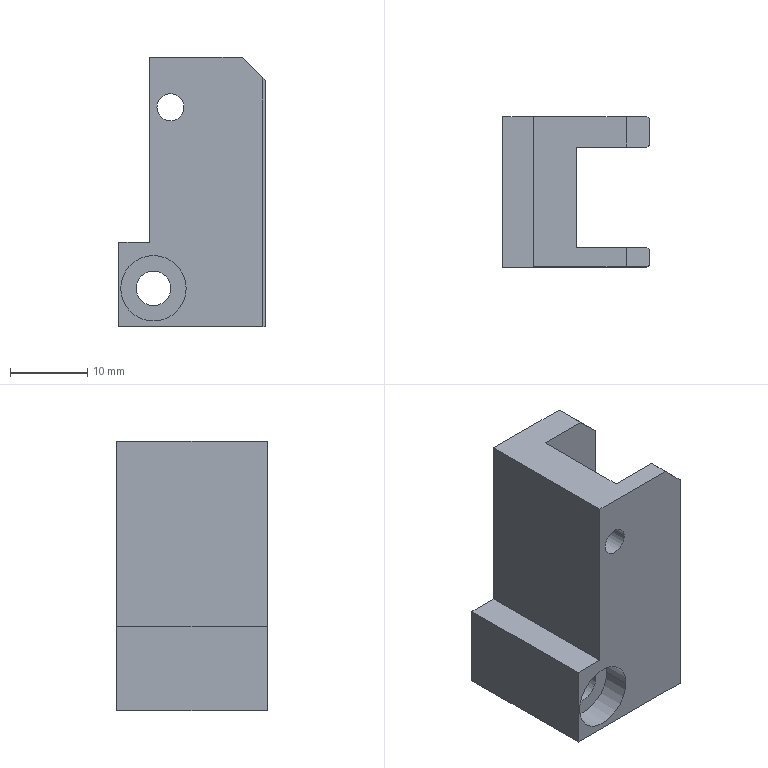Part | NX | 1 solid | 25 faces | box 19 x 19.5 x 35 mm | volume 6098 mm3 | plane 19 | cylinder 6 | commonest cylinder face diameters 3.5 x2 4.5 x2 8.5 x2
STEP:
#1=CARTESIAN_POINT('',(9.5,16.462,0.));
#2=VERTEX_POINT('',#1);
#3=CARTESIAN_POINT('',(18.7,16.462,0.));
#4=VERTEX_POINT('',#3);
#5=CARTESIAN_POINT('',(0.,16.462,0.));
#6=DIRECTION('',(1.,0.,0.));
#7=VECTOR('',#6,1000.);
#8=LINE('',#5,#7);
#9=EDGE_CURVE('',#2,#4,#8,.T.);
#10=ORIENTED_EDGE('',*,*,#9,.F.);
#11=CARTESIAN_POINT('',(9.5,3.462,0.));
#12=VERTEX_POINT('',#11);
#13=CARTESIAN_POINT('',(9.5,0.,0.));
#14=DIRECTION('',(0.,1.,0.));
#15=VECTOR('',#14,1000.);
#16=LINE('',#13,#15);
#17=EDGE_CURVE('',#12,#2,#16,.T.);
#18=ORIENTED_EDGE('',*,*,#17,.F.);
#19=CARTESIAN_POINT('',(18.7,3.462,0.));
#20=VERTEX_POINT('',#19);
#21=CARTESIAN_POINT('',(0.,3.462,0.));
#22=DIRECTION('',(-1.,0.,0.));
#23=VECTOR('',#22,1000.);
#24=LINE('',#21,#23);
#25=EDGE_CURVE('',#20,#12,#24,.T.);
#26=ORIENTED_EDGE('',*,*,#25,.F.);
#27=CARTESIAN_POINT('',(19.,3.162,0.));
#28=VERTEX_POINT('',#27);
#29=CARTESIAN_POINT('',(0.,22.162,0.));
#30=DIRECTION('',(0.7071,-0.7071,0.));
#31=VECTOR('',#30,1000.);
#32=LINE('',#29,#31);
#33=EDGE_CURVE('',#20,#28,#32,.T.);
#34=ORIENTED_EDGE('',*,*,#33,.T.);
#35=CARTESIAN_POINT('',(19.,1.212,0.));
#36=VERTEX_POINT('',#35);
#37=CARTESIAN_POINT('',(19.,0.,0.));
#38=DIRECTION('',(0.,-1.,0.));
#39=VECTOR('',#38,1000.);
#40=LINE('',#37,#39);
#41=EDGE_CURVE('',#28,#36,#40,.T.);
#42=ORIENTED_EDGE('',*,*,#41,.T.);
#43=CARTESIAN_POINT('',(18.7,0.912,0.));
#44=VERTEX_POINT('',#43);
#45=CARTESIAN_POINT('',(0.,-17.788,0.));
#46=DIRECTION('',(0.7071,0.7071,0.));
#47=VECTOR('',#46,1000.);
#48=LINE('',#45,#47);
#49=EDGE_CURVE('',#44,#36,#48,.T.);
#50=ORIENTED_EDGE('',*,*,#49,.F.);
#51=CARTESIAN_POINT('',(0.,0.912,0.));
#52=VERTEX_POINT('',#51);
#53=CARTESIAN_POINT('',(0.,0.912,0.));
#54=DIRECTION('',(-1.,0.,0.));
#55=VECTOR('',#54,1000.);
#56=LINE('',#53,#55);
#57=EDGE_CURVE('',#44,#52,#56,.T.);
#58=ORIENTED_EDGE('',*,*,#57,.T.);
#59=CARTESIAN_POINT('',(0.,20.412,0.));
#60=VERTEX_POINT('',#59);
#61=CARTESIAN_POINT('',(0.,0.,0.));
#62=DIRECTION('',(0.,-1.,0.));
#63=VECTOR('',#62,1000.);
#64=LINE('',#61,#63);
#65=EDGE_CURVE('',#60,#52,#64,.T.);
#66=ORIENTED_EDGE('',*,*,#65,.F.);
#67=CARTESIAN_POINT('',(18.7,20.412,0.));
#68=VERTEX_POINT('',#67);
#69=CARTESIAN_POINT('',(0.,20.412,0.));
#70=DIRECTION('',(-1.,0.,0.));
#71=VECTOR('',#70,1000.);
#72=LINE('',#69,#71);
#73=EDGE_CURVE('',#68,#60,#72,.T.);
#74=ORIENTED_EDGE('',*,*,#73,.F.);
#75=CARTESIAN_POINT('',(19.,20.112,0.));
#76=VERTEX_POINT('',#75);
#77=CARTESIAN_POINT('',(39.112,0.,0.));
#78=DIRECTION('',(-0.7071,0.7071,0.));
#79=VECTOR('',#78,1000.);
#80=LINE('',#77,#79);
#81=EDGE_CURVE('',#76,#68,#80,.T.);
#82=ORIENTED_EDGE('',*,*,#81,.F.);
#83=CARTESIAN_POINT('',(19.,16.762,0.));
#84=VERTEX_POINT('',#83);
#85=CARTESIAN_POINT('',(19.,0.,0.));
#86=DIRECTION('',(0.,1.,0.));
#87=VECTOR('',#86,1000.);
#88=LINE('',#85,#87);
#89=EDGE_CURVE('',#84,#76,#88,.T.);
#90=ORIENTED_EDGE('',*,*,#89,.F.);
#91=CARTESIAN_POINT('',(2.238,0.,0.));
#92=DIRECTION('',(0.7071,0.7071,0.));
#93=VECTOR('',#92,1000.);
#94=LINE('',#91,#93);
#95=EDGE_CURVE('',#4,#84,#94,.T.);
#96=ORIENTED_EDGE('',*,*,#95,.F.);
#97=EDGE_LOOP('',(#10,#18,#26,#34,#42,#50,#58,#66,#74,#82,#90,#96));
#98=FACE_BOUND('',#97,.T.);
#99=CARTESIAN_POINT('',(0.,0.,0.));
#100=DIRECTION('',(0.,0.,1.));
#101=DIRECTION('',(1.,0.,0.));
#102=AXIS2_PLACEMENT_3D('',#99,#100,#101);
#103=PLANE('',#102);
#104=ADVANCED_FACE('',(#98),#103,.F.);
#105=CARTESIAN_POINT('',(18.7,16.462,32.3));
#106=VERTEX_POINT('',#105);
#107=CARTESIAN_POINT('',(18.7,16.462,0.));
#108=DIRECTION('',(0.,0.,-1.));
#109=VECTOR('',#108,1000.);
#110=LINE('',#107,#109);
#111=EDGE_CURVE('',#106,#4,#110,.T.);
#112=ORIENTED_EDGE('',*,*,#111,.F.);
#113=CARTESIAN_POINT('',(16.,16.462,35.));
#114=VERTEX_POINT('',#113);
#115=CARTESIAN_POINT('',(51.,16.462,0.));
#116=DIRECTION('',(-0.7071,0.,0.7071));
#117=VECTOR('',#116,1000.);
#118=LINE('',#115,#117);
#119=EDGE_CURVE('',#106,#114,#118,.T.);
#120=ORIENTED_EDGE('',*,*,#119,.T.);
#121=CARTESIAN_POINT('',(9.5,16.462,35.));
#122=VERTEX_POINT('',#121);
#123=CARTESIAN_POINT('',(0.,16.462,35.));
#124=DIRECTION('',(1.,0.,0.));
#125=VECTOR('',#124,1000.);
#126=LINE('',#123,#125);
#127=EDGE_CURVE('',#122,#114,#126,.T.);
#128=ORIENTED_EDGE('',*,*,#127,.F.);
#129=CARTESIAN_POINT('',(9.5,16.462,0.));
#130=DIRECTION('',(0.,0.,1.));
#131=VECTOR('',#130,1000.);
#132=LINE('',#129,#131);
#133=EDGE_CURVE('',#2,#122,#132,.T.);
#134=ORIENTED_EDGE('',*,*,#133,.F.);
#135=ORIENTED_EDGE('',*,*,#9,.T.);
#136=EDGE_LOOP('',(#112,#120,#128,#134,#135));
#137=FACE_BOUND('',#136,.T.);
#138=CARTESIAN_POINT('',(19.,16.462,35.));
#139=DIRECTION('',(0.,1.,0.));
#140=DIRECTION('',(1.,0.,0.));
#141=AXIS2_PLACEMENT_3D('',#138,#139,#140);
#142=PLANE('',#141);
#143=ADVANCED_FACE('',(#137),#142,.F.);
#144=ORIENTED_EDGE('',*,*,#17,.T.);
#145=ORIENTED_EDGE('',*,*,#133,.T.);
#146=CARTESIAN_POINT('',(9.5,3.462,35.));
#147=VERTEX_POINT('',#146);
#148=CARTESIAN_POINT('',(9.5,0.,35.));
#149=DIRECTION('',(0.,1.,0.));
#150=VECTOR('',#149,1000.);
#151=LINE('',#148,#150);
#152=EDGE_CURVE('',#147,#122,#151,.T.);
#153=ORIENTED_EDGE('',*,*,#152,.F.);
#154=CARTESIAN_POINT('',(9.5,3.462,0.));
#155=DIRECTION('',(0.,0.,1.));
#156=VECTOR('',#155,1000.);
#157=LINE('',#154,#156);
#158=EDGE_CURVE('',#12,#147,#157,.T.);
#159=ORIENTED_EDGE('',*,*,#158,.F.);
#160=EDGE_LOOP('',(#144,#145,#153,#159));
#161=FACE_BOUND('',#160,.T.);
#162=CARTESIAN_POINT('',(9.5,16.95,35.));
#163=DIRECTION('',(-1.,0.,0.));
#164=DIRECTION('',(0.,0.,1.));
#165=AXIS2_PLACEMENT_3D('',#162,#163,#164);
#166=PLANE('',#165);
#167=ADVANCED_FACE('',(#161),#166,.F.);
#168=CARTESIAN_POINT('',(18.7,3.462,32.3));
#169=VERTEX_POINT('',#168);
#170=CARTESIAN_POINT('',(18.7,3.462,0.));
#171=DIRECTION('',(0.,0.,-1.));
#172=VECTOR('',#171,1000.);
#173=LINE('',#170,#172);
#174=EDGE_CURVE('',#169,#20,#173,.T.);
#175=ORIENTED_EDGE('',*,*,#174,.T.);
#176=ORIENTED_EDGE('',*,*,#25,.T.);
#177=ORIENTED_EDGE('',*,*,#158,.T.);
#178=CARTESIAN_POINT('',(16.,3.462,35.));
#179=VERTEX_POINT('',#178);
#180=CARTESIAN_POINT('',(0.,3.462,35.));
#181=DIRECTION('',(-1.,0.,0.));
#182=VECTOR('',#181,1000.);
#183=LINE('',#180,#182);
#184=EDGE_CURVE('',#179,#147,#183,.T.);
#185=ORIENTED_EDGE('',*,*,#184,.F.);
#186=CARTESIAN_POINT('',(51.,3.462,0.));
#187=DIRECTION('',(0.7071,0.,-0.7071));
#188=VECTOR('',#187,1000.);
#189=LINE('',#186,#188);
#190=EDGE_CURVE('',#179,#169,#189,.T.);
#191=ORIENTED_EDGE('',*,*,#190,.T.);
#192=EDGE_LOOP('',(#175,#176,#177,#185,#191));
#193=FACE_BOUND('',#192,.T.);
#194=CARTESIAN_POINT('',(9.5,3.462,35.));
#195=DIRECTION('',(0.,-1.,0.));
#196=DIRECTION('',(0.,0.,-1.));
#197=AXIS2_PLACEMENT_3D('',#194,#195,#196);
#198=PLANE('',#197);
#199=ADVANCED_FACE('',(#193),#198,.F.);
#200=CARTESIAN_POINT('',(19.,3.162,32.));
#201=VERTEX_POINT('',#200);
#202=CARTESIAN_POINT('',(19.,3.162,0.));
#203=DIRECTION('',(0.,0.,-1.));
#204=VECTOR('',#203,1000.);
#205=LINE('',#202,#204);
#206=EDGE_CURVE('',#201,#28,#205,.T.);
#207=ORIENTED_EDGE('',*,*,#206,.F.);
#208=CARTESIAN_POINT('',(19.,1.212,32.));
#209=VERTEX_POINT('',#208);
#210=CARTESIAN_POINT('',(19.,0.,32.));
#211=DIRECTION('',(0.,1.,0.));
#212=VECTOR('',#211,1000.);
#213=LINE('',#210,#212);
#214=EDGE_CURVE('',#209,#201,#213,.T.);
#215=ORIENTED_EDGE('',*,*,#214,.F.);
#216=CARTESIAN_POINT('',(19.,1.212,0.));
#217=DIRECTION('',(0.,0.,-1.));
#218=VECTOR('',#217,1000.);
#219=LINE('',#216,#218);
#220=EDGE_CURVE('',#209,#36,#219,.T.);
#221=ORIENTED_EDGE('',*,*,#220,.T.);
#222=ORIENTED_EDGE('',*,*,#41,.F.);
#223=EDGE_LOOP('',(#207,#215,#221,#222));
#224=FACE_BOUND('',#223,.T.);
#225=CARTESIAN_POINT('',(19.,0.,0.));
#226=DIRECTION('',(1.,0.,0.));
#227=DIRECTION('',(0.,1.,0.));
#228=AXIS2_PLACEMENT_3D('',#225,#226,#227);
#229=PLANE('',#228);
#230=ADVANCED_FACE('',(#224),#229,.T.);
#231=CARTESIAN_POINT('',(0.25,4.4,5.));
#232=VERTEX_POINT('',#231);
#233=CARTESIAN_POINT('',(8.75,4.4,5.));
#234=VERTEX_POINT('',#233);
#235=CARTESIAN_POINT('',(4.5,4.4,5.));
#236=DIRECTION('',(0.,-1.,0.));
#237=DIRECTION('',(-1.,0.,0.));
#238=AXIS2_PLACEMENT_3D('',#235,#236,#237);
#239=CIRCLE('',#238,4.25);
#240=EDGE_CURVE('',#232,#234,#239,.T.);
#241=ORIENTED_EDGE('',*,*,#240,.T.);
#242=CARTESIAN_POINT('',(4.5,4.4,5.));
#243=DIRECTION('',(0.,-1.,0.));
#244=DIRECTION('',(-1.,0.,0.));
#245=AXIS2_PLACEMENT_3D('',#242,#243,#244);
#246=CIRCLE('',#245,4.25);
#247=EDGE_CURVE('',#234,#232,#246,.T.);
#248=ORIENTED_EDGE('',*,*,#247,.T.);
#249=EDGE_LOOP('',(#241,#248));
#250=FACE_BOUND('',#249,.T.);
#251=CARTESIAN_POINT('',(6.75,4.4,5.));
#252=VERTEX_POINT('',#251);
#253=CARTESIAN_POINT('',(2.25,4.4,5.));
#254=VERTEX_POINT('',#253);
#255=CARTESIAN_POINT('',(4.5,4.4,5.));
#256=DIRECTION('',(0.,-1.,0.));
#257=DIRECTION('',(1.,0.,0.));
#258=AXIS2_PLACEMENT_3D('',#255,#256,#257);
#259=CIRCLE('',#258,2.25);
#260=EDGE_CURVE('',#252,#254,#259,.T.);
#261=ORIENTED_EDGE('',*,*,#260,.F.);
#262=CARTESIAN_POINT('',(4.5,4.4,5.));
#263=DIRECTION('',(0.,-1.,0.));
#264=DIRECTION('',(1.,0.,0.));
#265=AXIS2_PLACEMENT_3D('',#262,#263,#264);
#266=CIRCLE('',#265,2.25);
#267=EDGE_CURVE('',#254,#252,#266,.T.);
#268=ORIENTED_EDGE('',*,*,#267,.F.);
#269=EDGE_LOOP('',(#261,#268));
#270=FACE_BOUND('',#269,.T.);
#271=CARTESIAN_POINT('',(9.199,4.4,2.964));
#272=DIRECTION('',(0.,-1.,0.));
#273=DIRECTION('',(0.,0.,-1.));
#274=AXIS2_PLACEMENT_3D('',#271,#272,#273);
#275=PLANE('',#274);
#276=ADVANCED_FACE('',(#250,#270),#275,.T.);
#277=CARTESIAN_POINT('',(4.,20.412,35.));
#278=VERTEX_POINT('',#277);
#279=CARTESIAN_POINT('',(4.,0.912,35.));
#280=VERTEX_POINT('',#279);
#281=CARTESIAN_POINT('',(4.,0.,35.));
#282=DIRECTION('',(0.,-1.,0.));
#283=VECTOR('',#282,1000.);
#284=LINE('',#281,#283);
#285=EDGE_CURVE('',#278,#280,#284,.T.);
#286=ORIENTED_EDGE('',*,*,#285,.F.);
#287=CARTESIAN_POINT('',(4.,20.412,11.));
#288=VERTEX_POINT('',#287);
#289=CARTESIAN_POINT('',(4.,20.412,0.));
#290=DIRECTION('',(0.,0.,1.));
#291=VECTOR('',#290,1000.);
#292=LINE('',#289,#291);
#293=EDGE_CURVE('',#288,#278,#292,.T.);
#294=ORIENTED_EDGE('',*,*,#293,.F.);
#295=CARTESIAN_POINT('',(4.,0.912,11.));
#296=VERTEX_POINT('',#295);
#297=CARTESIAN_POINT('',(4.,0.,11.));
#298=DIRECTION('',(0.,-1.,0.));
#299=VECTOR('',#298,1000.);
#300=LINE('',#297,#299);
#301=EDGE_CURVE('',#288,#296,#300,.T.);
#302=ORIENTED_EDGE('',*,*,#301,.T.);
#303=CARTESIAN_POINT('',(4.,0.912,0.));
#304=DIRECTION('',(0.,0.,1.));
#305=VECTOR('',#304,1000.);
#306=LINE('',#303,#305);
#307=EDGE_CURVE('',#296,#280,#306,.T.);
#308=ORIENTED_EDGE('',*,*,#307,.T.);
#309=EDGE_LOOP('',(#286,#294,#302,#308));
#310=FACE_BOUND('',#309,.T.);
#311=CARTESIAN_POINT('',(4.,20.5,35.));
#312=DIRECTION('',(1.,0.,0.));
#313=DIRECTION('',(0.,1.,0.));
#314=AXIS2_PLACEMENT_3D('',#311,#312,#313);
#315=PLANE('',#314);
#316=ADVANCED_FACE('',(#310),#315,.F.);
#317=ORIENTED_EDGE('',*,*,#285,.T.);
#318=CARTESIAN_POINT('',(16.,0.912,35.));
#319=VERTEX_POINT('',#318);
#320=CARTESIAN_POINT('',(0.,0.912,35.));
#321=DIRECTION('',(-1.,0.,0.));
#322=VECTOR('',#321,1000.);
#323=LINE('',#320,#322);
#324=EDGE_CURVE('',#319,#280,#323,.T.);
#325=ORIENTED_EDGE('',*,*,#324,.F.);
#326=CARTESIAN_POINT('',(16.,0.,35.));
#327=DIRECTION('',(0.,1.,0.));
#328=VECTOR('',#327,1000.);
#329=LINE('',#326,#328);
#330=EDGE_CURVE('',#319,#179,#329,.T.);
#331=ORIENTED_EDGE('',*,*,#330,.T.);
#332=ORIENTED_EDGE('',*,*,#184,.T.);
#333=ORIENTED_EDGE('',*,*,#152,.T.);
#334=ORIENTED_EDGE('',*,*,#127,.T.);
#335=CARTESIAN_POINT('',(16.,20.412,35.));
#336=VERTEX_POINT('',#335);
#337=CARTESIAN_POINT('',(16.,0.,35.));
#338=DIRECTION('',(0.,1.,0.));
#339=VECTOR('',#338,1000.);
#340=LINE('',#337,#339);
#341=EDGE_CURVE('',#114,#336,#340,.T.);
#342=ORIENTED_EDGE('',*,*,#341,.T.);
#343=CARTESIAN_POINT('',(0.,20.412,35.));
#344=DIRECTION('',(1.,0.,0.));
#345=VECTOR('',#344,1000.);
#346=LINE('',#343,#345);
#347=EDGE_CURVE('',#278,#336,#346,.T.);
#348=ORIENTED_EDGE('',*,*,#347,.F.);
#349=EDGE_LOOP('',(#317,#325,#331,#332,#333,#334,#342,#348));
#350=FACE_BOUND('',#349,.T.);
#351=CARTESIAN_POINT('',(0.,0.,35.));
#352=DIRECTION('',(0.,0.,1.));
#353=DIRECTION('',(1.,0.,0.));
#354=AXIS2_PLACEMENT_3D('',#351,#352,#353);
#355=PLANE('',#354);
#356=ADVANCED_FACE('',(#350),#355,.T.);
#357=CARTESIAN_POINT('',(18.7,0.912,32.3));
#358=VERTEX_POINT('',#357);
#359=CARTESIAN_POINT('',(18.7,0.912,0.));
#360=DIRECTION('',(0.,0.,1.));
#361=VECTOR('',#360,1000.);
#362=LINE('',#359,#361);
#363=EDGE_CURVE('',#44,#358,#362,.T.);
#364=ORIENTED_EDGE('',*,*,#363,.T.);
#365=CARTESIAN_POINT('',(51.,0.912,0.));
#366=DIRECTION('',(0.7071,0.,-0.7071));
#367=VECTOR('',#366,1000.);
#368=LINE('',#365,#367);
#369=EDGE_CURVE('',#319,#358,#368,.T.);
#370=ORIENTED_EDGE('',*,*,#369,.F.);
#371=ORIENTED_EDGE('',*,*,#324,.T.);
#372=ORIENTED_EDGE('',*,*,#307,.F.);
#373=CARTESIAN_POINT('',(0.,0.912,11.));
#374=VERTEX_POINT('',#373);
#375=CARTESIAN_POINT('',(0.,0.912,11.));
#376=DIRECTION('',(1.,0.,0.));
#377=VECTOR('',#376,1000.);
#378=LINE('',#375,#377);
#379=EDGE_CURVE('',#374,#296,#378,.T.);
#380=ORIENTED_EDGE('',*,*,#379,.F.);
#381=CARTESIAN_POINT('',(0.,0.912,0.));
#382=DIRECTION('',(0.,0.,-1.));
#383=VECTOR('',#382,1000.);
#384=LINE('',#381,#383);
#385=EDGE_CURVE('',#374,#52,#384,.T.);
#386=ORIENTED_EDGE('',*,*,#385,.T.);
#387=ORIENTED_EDGE('',*,*,#57,.F.);
#388=EDGE_LOOP('',(#364,#370,#371,#372,#380,#386,#387));
#389=FACE_BOUND('',#388,.T.);
#390=CARTESIAN_POINT('',(8.45,0.912,28.5));
#391=VERTEX_POINT('',#390);
#392=CARTESIAN_POINT('',(4.95,0.912,28.5));
#393=VERTEX_POINT('',#392);
#394=CARTESIAN_POINT('',(6.7,0.912,28.5));
#395=DIRECTION('',(0.,-1.,0.));
#396=DIRECTION('',(1.,0.,0.));
#397=AXIS2_PLACEMENT_3D('',#394,#395,#396);
#398=CIRCLE('',#397,1.75);
#399=EDGE_CURVE('',#391,#393,#398,.T.);
#400=ORIENTED_EDGE('',*,*,#399,.F.);
#401=CARTESIAN_POINT('',(6.7,0.912,28.5));
#402=DIRECTION('',(0.,-1.,0.));
#403=DIRECTION('',(1.,0.,0.));
#404=AXIS2_PLACEMENT_3D('',#401,#402,#403);
#405=CIRCLE('',#404,1.75);
#406=EDGE_CURVE('',#393,#391,#405,.T.);
#407=ORIENTED_EDGE('',*,*,#406,.F.);
#408=EDGE_LOOP('',(#400,#407));
#409=FACE_BOUND('',#408,.T.);
#410=CARTESIAN_POINT('',(8.75,0.912,5.));
#411=VERTEX_POINT('',#410);
#412=CARTESIAN_POINT('',(0.25,0.912,5.));
#413=VERTEX_POINT('',#412);
#414=CARTESIAN_POINT('',(4.5,0.912,5.));
#415=DIRECTION('',(0.,-1.,0.));
#416=DIRECTION('',(-1.,0.,0.));
#417=AXIS2_PLACEMENT_3D('',#414,#415,#416);
#418=CIRCLE('',#417,4.25);
#419=EDGE_CURVE('',#411,#413,#418,.T.);
#420=ORIENTED_EDGE('',*,*,#419,.F.);
#421=CARTESIAN_POINT('',(4.5,0.912,5.));
#422=DIRECTION('',(0.,-1.,0.));
#423=DIRECTION('',(-1.,0.,0.));
#424=AXIS2_PLACEMENT_3D('',#421,#422,#423);
#425=CIRCLE('',#424,4.25);
#426=EDGE_CURVE('',#413,#411,#425,.T.);
#427=ORIENTED_EDGE('',*,*,#426,.F.);
#428=EDGE_LOOP('',(#420,#427));
#429=FACE_BOUND('',#428,.T.);
#430=CARTESIAN_POINT('',(0.,0.912,0.));
#431=DIRECTION('',(0.,-1.,0.));
#432=DIRECTION('',(0.,0.,-1.));
#433=AXIS2_PLACEMENT_3D('',#430,#431,#432);
#434=PLANE('',#433);
#435=ADVANCED_FACE('',(#389,#409,#429),#434,.T.);
#436=ORIENTED_EDGE('',*,*,#379,.T.);
#437=ORIENTED_EDGE('',*,*,#301,.F.);
#438=CARTESIAN_POINT('',(0.,20.412,11.));
#439=VERTEX_POINT('',#438);
#440=CARTESIAN_POINT('',(0.,20.412,11.));
#441=DIRECTION('',(1.,0.,0.));
#442=VECTOR('',#441,1000.);
#443=LINE('',#440,#442);
#444=EDGE_CURVE('',#439,#288,#443,.T.);
#445=ORIENTED_EDGE('',*,*,#444,.F.);
#446=CARTESIAN_POINT('',(0.,0.,11.));
#447=DIRECTION('',(0.,1.,0.));
#448=VECTOR('',#447,1000.);
#449=LINE('',#446,#448);
#450=EDGE_CURVE('',#374,#439,#449,.T.);
#451=ORIENTED_EDGE('',*,*,#450,.F.);
#452=EDGE_LOOP('',(#436,#437,#445,#451));
#453=FACE_BOUND('',#452,.T.);
#454=CARTESIAN_POINT('',(4.,20.5,11.));
#455=DIRECTION('',(0.,0.,-1.));
#456=DIRECTION('',(0.,-1.,0.));
#457=AXIS2_PLACEMENT_3D('',#454,#455,#456);
#458=PLANE('',#457);
#459=ADVANCED_FACE('',(#453),#458,.F.);
#460=ORIENTED_EDGE('',*,*,#450,.T.);
#461=CARTESIAN_POINT('',(0.,20.412,0.));
#462=DIRECTION('',(0.,0.,1.));
#463=VECTOR('',#462,1000.);
#464=LINE('',#461,#463);
#465=EDGE_CURVE('',#60,#439,#464,.T.);
#466=ORIENTED_EDGE('',*,*,#465,.F.);
#467=ORIENTED_EDGE('',*,*,#65,.T.);
#468=ORIENTED_EDGE('',*,*,#385,.F.);
#469=EDGE_LOOP('',(#460,#466,#467,#468));
#470=FACE_BOUND('',#469,.T.);
#471=CARTESIAN_POINT('',(0.,20.5,0.));
#472=DIRECTION('',(-1.,0.,0.));
#473=DIRECTION('',(0.,0.,1.));
#474=AXIS2_PLACEMENT_3D('',#471,#472,#473);
#475=PLANE('',#474);
#476=ADVANCED_FACE('',(#470),#475,.T.);
#477=CARTESIAN_POINT('',(19.,16.762,32.));
#478=VERTEX_POINT('',#477);
#479=CARTESIAN_POINT('',(19.,16.762,0.));
#480=DIRECTION('',(0.,0.,-1.));
#481=VECTOR('',#480,1000.);
#482=LINE('',#479,#481);
#483=EDGE_CURVE('',#478,#84,#482,.T.);
#484=ORIENTED_EDGE('',*,*,#483,.T.);
#485=ORIENTED_EDGE('',*,*,#89,.T.);
#486=CARTESIAN_POINT('',(19.,20.112,32.));
#487=VERTEX_POINT('',#486);
#488=CARTESIAN_POINT('',(19.,20.112,0.));
#489=DIRECTION('',(0.,0.,1.));
#490=VECTOR('',#489,1000.);
#491=LINE('',#488,#490);
#492=EDGE_CURVE('',#76,#487,#491,.T.);
#493=ORIENTED_EDGE('',*,*,#492,.T.);
#494=CARTESIAN_POINT('',(19.,0.,32.));
#495=DIRECTION('',(0.,-1.,0.));
#496=VECTOR('',#495,1000.);
#497=LINE('',#494,#496);
#498=EDGE_CURVE('',#487,#478,#497,.T.);
#499=ORIENTED_EDGE('',*,*,#498,.T.);
#500=EDGE_LOOP('',(#484,#485,#493,#499));
#501=FACE_BOUND('',#500,.T.);
#502=CARTESIAN_POINT('',(19.,0.,0.));
#503=DIRECTION('',(1.,0.,0.));
#504=DIRECTION('',(0.,1.,0.));
#505=AXIS2_PLACEMENT_3D('',#502,#503,#504);
#506=PLANE('',#505);
#507=ADVANCED_FACE('',(#501),#506,.T.);
#508=ORIENTED_EDGE('',*,*,#341,.F.);
#509=ORIENTED_EDGE('',*,*,#119,.F.);
#510=CARTESIAN_POINT('',(51.,48.762,0.));
#511=DIRECTION('',(-0.5774,-0.5774,0.5774));
#512=VECTOR('',#511,1000.);
#513=LINE('',#510,#512);
#514=EDGE_CURVE('',#478,#106,#513,.T.);
#515=ORIENTED_EDGE('',*,*,#514,.F.);
#516=ORIENTED_EDGE('',*,*,#498,.F.);
#517=CARTESIAN_POINT('',(18.7,20.412,32.3));
#518=VERTEX_POINT('',#517);
#519=CARTESIAN_POINT('',(51.,-11.888,0.));
#520=DIRECTION('',(0.5774,-0.5774,-0.5774));
#521=VECTOR('',#520,1000.);
#522=LINE('',#519,#521);
#523=EDGE_CURVE('',#518,#487,#522,.T.);
#524=ORIENTED_EDGE('',*,*,#523,.F.);
#525=CARTESIAN_POINT('',(51.,20.412,0.));
#526=DIRECTION('',(-0.7071,0.,0.7071));
#527=VECTOR('',#526,1000.);
#528=LINE('',#525,#527);
#529=EDGE_CURVE('',#518,#336,#528,.T.);
#530=ORIENTED_EDGE('',*,*,#529,.T.);
#531=EDGE_LOOP('',(#508,#509,#515,#516,#524,#530));
#532=FACE_BOUND('',#531,.T.);
#533=CARTESIAN_POINT('',(16.,16.95,35.));
#534=DIRECTION('',(-0.7071,0.,-0.7071));
#535=DIRECTION('',(-0.7071,0.,0.7071));
#536=AXIS2_PLACEMENT_3D('',#533,#534,#535);
#537=PLANE('',#536);
#538=ADVANCED_FACE('',(#532),#537,.F.);
#539=ORIENTED_EDGE('',*,*,#399,.T.);
#540=CARTESIAN_POINT('',(4.95,20.412,28.5));
#541=VERTEX_POINT('',#540);
#542=CARTESIAN_POINT('',(4.95,20.5,28.5));
#543=DIRECTION('',(0.,-1.,0.));
#544=VECTOR('',#543,1000.);
#545=LINE('',#542,#544);
#546=EDGE_CURVE('',#393,#541,#545,.F.);
#547=ORIENTED_EDGE('',*,*,#546,.T.);
#548=CARTESIAN_POINT('',(8.45,20.412,28.5));
#549=VERTEX_POINT('',#548);
#550=CARTESIAN_POINT('',(6.7,20.412,28.5));
#551=DIRECTION('',(0.,-1.,0.));
#552=DIRECTION('',(1.,0.,0.));
#553=AXIS2_PLACEMENT_3D('',#550,#551,#552);
#554=CIRCLE('',#553,1.75);
#555=EDGE_CURVE('',#549,#541,#554,.T.);
#556=ORIENTED_EDGE('',*,*,#555,.F.);
#557=CARTESIAN_POINT('',(8.45,20.5,28.5));
#558=DIRECTION('',(0.,-1.,0.));
#559=VECTOR('',#558,1000.);
#560=LINE('',#557,#559);
#561=EDGE_CURVE('',#391,#549,#560,.F.);
#562=ORIENTED_EDGE('',*,*,#561,.F.);
#563=EDGE_LOOP('',(#539,#547,#556,#562));
#564=FACE_BOUND('',#563,.T.);
#565=CARTESIAN_POINT('',(6.7,20.5,28.5));
#566=DIRECTION('',(0.,-1.,0.));
#567=DIRECTION('',(1.,0.,0.));
#568=AXIS2_PLACEMENT_3D('',#565,#566,#567);
#569=CYLINDRICAL_SURFACE('',#568,1.75);
#570=ADVANCED_FACE('',(#564),#569,.F.);
#571=ORIENTED_EDGE('',*,*,#330,.F.);
#572=ORIENTED_EDGE('',*,*,#369,.T.);
#573=CARTESIAN_POINT('',(51.,33.212,0.));
#574=DIRECTION('',(-0.5774,-0.5774,0.5774));
#575=VECTOR('',#574,1000.);
#576=LINE('',#573,#575);
#577=EDGE_CURVE('',#209,#358,#576,.T.);
#578=ORIENTED_EDGE('',*,*,#577,.F.);
#579=ORIENTED_EDGE('',*,*,#214,.T.);
#580=CARTESIAN_POINT('',(51.,-28.838,0.));
#581=DIRECTION('',(-0.5774,0.5774,0.5774));
#582=VECTOR('',#581,1000.);
#583=LINE('',#580,#582);
#584=EDGE_CURVE('',#201,#169,#583,.T.);
#585=ORIENTED_EDGE('',*,*,#584,.T.);
#586=ORIENTED_EDGE('',*,*,#190,.F.);
#587=EDGE_LOOP('',(#571,#572,#578,#579,#585,#586));
#588=FACE_BOUND('',#587,.T.);
#589=CARTESIAN_POINT('',(16.,0.,35.));
#590=DIRECTION('',(-0.7071,0.,-0.7071));
#591=DIRECTION('',(-0.7071,0.,0.7071));
#592=AXIS2_PLACEMENT_3D('',#589,#590,#591);
#593=PLANE('',#592);
#594=ADVANCED_FACE('',(#588),#593,.F.);
#595=CARTESIAN_POINT('',(2.25,20.412,5.));
#596=VERTEX_POINT('',#595);
#597=CARTESIAN_POINT('',(6.75,20.412,5.));
#598=VERTEX_POINT('',#597);
#599=CARTESIAN_POINT('',(4.5,20.412,5.));
#600=DIRECTION('',(0.,-1.,0.));
#601=DIRECTION('',(1.,0.,0.));
#602=AXIS2_PLACEMENT_3D('',#599,#600,#601);
#603=CIRCLE('',#602,2.25);
#604=EDGE_CURVE('',#596,#598,#603,.T.);
#605=ORIENTED_EDGE('',*,*,#604,.F.);
#606=CARTESIAN_POINT('',(2.25,20.5,5.));
#607=DIRECTION('',(0.,-1.,0.));
#608=VECTOR('',#607,1000.);
#609=LINE('',#606,#608);
#610=EDGE_CURVE('',#254,#596,#609,.F.);
#611=ORIENTED_EDGE('',*,*,#610,.F.);
#612=ORIENTED_EDGE('',*,*,#267,.T.);
#613=CARTESIAN_POINT('',(6.75,20.5,5.));
#614=DIRECTION('',(0.,-1.,0.));
#615=VECTOR('',#614,1000.);
#616=LINE('',#613,#615);
#617=EDGE_CURVE('',#252,#598,#616,.F.);
#618=ORIENTED_EDGE('',*,*,#617,.T.);
#619=EDGE_LOOP('',(#605,#611,#612,#618));
#620=FACE_BOUND('',#619,.T.);
#621=CARTESIAN_POINT('',(4.5,20.5,5.));
#622=DIRECTION('',(0.,-1.,0.));
#623=DIRECTION('',(1.,0.,0.));
#624=AXIS2_PLACEMENT_3D('',#621,#622,#623);
#625=CYLINDRICAL_SURFACE('',#624,2.25);
#626=ADVANCED_FACE('',(#620),#625,.F.);
#627=ORIENTED_EDGE('',*,*,#419,.T.);
#628=CARTESIAN_POINT('',(0.25,0.9,5.));
#629=DIRECTION('',(0.,-1.,0.));
#630=VECTOR('',#629,1000.);
#631=LINE('',#628,#630);
#632=EDGE_CURVE('',#413,#232,#631,.F.);
#633=ORIENTED_EDGE('',*,*,#632,.T.);
#634=ORIENTED_EDGE('',*,*,#247,.F.);
#635=CARTESIAN_POINT('',(8.75,0.9,5.));
#636=DIRECTION('',(0.,-1.,0.));
#637=VECTOR('',#636,1000.);
#638=LINE('',#635,#637);
#639=EDGE_CURVE('',#411,#234,#638,.F.);
#640=ORIENTED_EDGE('',*,*,#639,.F.);
#641=EDGE_LOOP('',(#627,#633,#634,#640));
#642=FACE_BOUND('',#641,.T.);
#643=CARTESIAN_POINT('',(4.5,0.9,5.));
#644=DIRECTION('',(0.,-1.,0.));
#645=DIRECTION('',(-1.,0.,0.));
#646=AXIS2_PLACEMENT_3D('',#643,#644,#645);
#647=CYLINDRICAL_SURFACE('',#646,4.25);
#648=ADVANCED_FACE('',(#642),#647,.F.);
#649=CARTESIAN_POINT('',(18.7,20.412,0.));
#650=DIRECTION('',(0.,0.,-1.));
#651=VECTOR('',#650,1000.);
#652=LINE('',#649,#651);
#653=EDGE_CURVE('',#518,#68,#652,.T.);
#654=ORIENTED_EDGE('',*,*,#653,.T.);
#655=ORIENTED_EDGE('',*,*,#73,.T.);
#656=ORIENTED_EDGE('',*,*,#465,.T.);
#657=ORIENTED_EDGE('',*,*,#444,.T.);
#658=ORIENTED_EDGE('',*,*,#293,.T.);
#659=ORIENTED_EDGE('',*,*,#347,.T.);
#660=ORIENTED_EDGE('',*,*,#529,.F.);
#661=EDGE_LOOP('',(#654,#655,#656,#657,#658,#659,#660));
#662=FACE_BOUND('',#661,.T.);
#663=CARTESIAN_POINT('',(6.7,20.412,28.5));
#664=DIRECTION('',(0.,-1.,0.));
#665=DIRECTION('',(1.,0.,0.));
#666=AXIS2_PLACEMENT_3D('',#663,#664,#665);
#667=CIRCLE('',#666,1.75);
#668=EDGE_CURVE('',#541,#549,#667,.T.);
#669=ORIENTED_EDGE('',*,*,#668,.T.);
#670=ORIENTED_EDGE('',*,*,#555,.T.);
#671=EDGE_LOOP('',(#669,#670));
#672=FACE_BOUND('',#671,.T.);
#673=ORIENTED_EDGE('',*,*,#604,.T.);
#674=CARTESIAN_POINT('',(4.5,20.412,5.));
#675=DIRECTION('',(0.,-1.,0.));
#676=DIRECTION('',(1.,0.,0.));
#677=AXIS2_PLACEMENT_3D('',#674,#675,#676);
#678=CIRCLE('',#677,2.25);
#679=EDGE_CURVE('',#598,#596,#678,.T.);
#680=ORIENTED_EDGE('',*,*,#679,.T.);
#681=EDGE_LOOP('',(#673,#680));
#682=FACE_BOUND('',#681,.T.);
#683=CARTESIAN_POINT('',(19.,20.412,0.));
#684=DIRECTION('',(0.,1.,0.));
#685=DIRECTION('',(1.,0.,0.));
#686=AXIS2_PLACEMENT_3D('',#683,#684,#685);
#687=PLANE('',#686);
#688=ADVANCED_FACE('',(#662,#672,#682),#687,.T.);
#689=ORIENTED_EDGE('',*,*,#111,.T.);
#690=ORIENTED_EDGE('',*,*,#95,.T.);
#691=ORIENTED_EDGE('',*,*,#483,.F.);
#692=ORIENTED_EDGE('',*,*,#514,.T.);
#693=EDGE_LOOP('',(#689,#690,#691,#692));
#694=FACE_BOUND('',#693,.T.);
#695=CARTESIAN_POINT('',(18.85,16.612,16.));
#696=DIRECTION('',(-0.7071,0.7071,0.));
#697=DIRECTION('',(0.,0.,1.));
#698=AXIS2_PLACEMENT_3D('',#695,#696,#697);
#699=PLANE('',#698);
#700=ADVANCED_FACE('',(#694),#699,.F.);
#701=ORIENTED_EDGE('',*,*,#363,.F.);
#702=ORIENTED_EDGE('',*,*,#49,.T.);
#703=ORIENTED_EDGE('',*,*,#220,.F.);
#704=ORIENTED_EDGE('',*,*,#577,.T.);
#705=EDGE_LOOP('',(#701,#702,#703,#704));
#706=FACE_BOUND('',#705,.T.);
#707=CARTESIAN_POINT('',(18.85,1.062,16.));
#708=DIRECTION('',(-0.7071,0.7071,0.));
#709=DIRECTION('',(0.,0.,1.));
#710=AXIS2_PLACEMENT_3D('',#707,#708,#709);
#711=PLANE('',#710);
#712=ADVANCED_FACE('',(#706),#711,.F.);
#713=ORIENTED_EDGE('',*,*,#174,.F.);
#714=ORIENTED_EDGE('',*,*,#584,.F.);
#715=ORIENTED_EDGE('',*,*,#206,.T.);
#716=ORIENTED_EDGE('',*,*,#33,.F.);
#717=EDGE_LOOP('',(#713,#714,#715,#716));
#718=FACE_BOUND('',#717,.T.);
#719=CARTESIAN_POINT('',(18.85,3.312,16.));
#720=DIRECTION('',(0.7071,0.7071,0.));
#721=DIRECTION('',(0.,0.,-1.));
#722=AXIS2_PLACEMENT_3D('',#719,#720,#721);
#723=PLANE('',#722);
#724=ADVANCED_FACE('',(#718),#723,.T.);
#725=ORIENTED_EDGE('',*,*,#653,.F.);
#726=ORIENTED_EDGE('',*,*,#523,.T.);
#727=ORIENTED_EDGE('',*,*,#492,.F.);
#728=ORIENTED_EDGE('',*,*,#81,.T.);
#729=EDGE_LOOP('',(#725,#726,#727,#728));
#730=FACE_BOUND('',#729,.T.);
#731=CARTESIAN_POINT('',(18.85,20.262,16.));
#732=DIRECTION('',(0.7071,0.7071,0.));
#733=DIRECTION('',(0.,0.,-1.));
#734=AXIS2_PLACEMENT_3D('',#731,#732,#733);
#735=PLANE('',#734);
#736=ADVANCED_FACE('',(#730),#735,.T.);
#737=ORIENTED_EDGE('',*,*,#260,.T.);
#738=ORIENTED_EDGE('',*,*,#610,.T.);
#739=ORIENTED_EDGE('',*,*,#679,.F.);
#740=ORIENTED_EDGE('',*,*,#617,.F.);
#741=EDGE_LOOP('',(#737,#738,#739,#740));
#742=FACE_BOUND('',#741,.T.);
#743=CARTESIAN_POINT('',(4.5,20.5,5.));
#744=DIRECTION('',(0.,-1.,0.));
#745=DIRECTION('',(1.,0.,0.));
#746=AXIS2_PLACEMENT_3D('',#743,#744,#745);
#747=CYLINDRICAL_SURFACE('',#746,2.25);
#748=ADVANCED_FACE('',(#742),#747,.F.);
#749=ORIENTED_EDGE('',*,*,#240,.F.);
#750=ORIENTED_EDGE('',*,*,#632,.F.);
#751=ORIENTED_EDGE('',*,*,#426,.T.);
#752=ORIENTED_EDGE('',*,*,#639,.T.);
#753=EDGE_LOOP('',(#749,#750,#751,#752));
#754=FACE_BOUND('',#753,.T.);
#755=CARTESIAN_POINT('',(4.5,0.9,5.));
#756=DIRECTION('',(0.,-1.,0.));
#757=DIRECTION('',(-1.,0.,0.));
#758=AXIS2_PLACEMENT_3D('',#755,#756,#757);
#759=CYLINDRICAL_SURFACE('',#758,4.25);
#760=ADVANCED_FACE('',(#754),#759,.F.);
#761=ORIENTED_EDGE('',*,*,#668,.F.);
#762=ORIENTED_EDGE('',*,*,#546,.F.);
#763=ORIENTED_EDGE('',*,*,#406,.T.);
#764=ORIENTED_EDGE('',*,*,#561,.T.);
#765=EDGE_LOOP('',(#761,#762,#763,#764));
#766=FACE_BOUND('',#765,.T.);
#767=CARTESIAN_POINT('',(6.7,20.5,28.5));
#768=DIRECTION('',(0.,-1.,0.));
#769=DIRECTION('',(1.,0.,0.));
#770=AXIS2_PLACEMENT_3D('',#767,#768,#769);
#771=CYLINDRICAL_SURFACE('',#770,1.75);
#772=ADVANCED_FACE('',(#766),#771,.F.);
#773=CLOSED_SHELL('',(#104,#143,#167,#199,#230,#276,#316,#356,#435,#459,#476,#507,#538,#570,#594,#626,#648,#688,#700,#712,#724,#736,#748,#760,#772));
#774=MANIFOLD_SOLID_BREP('',#773);
#775=(LENGTH_UNIT()NAMED_UNIT(*)SI_UNIT(.MILLI.,.METRE.));
#776=UNCERTAINTY_MEASURE_WITH_UNIT(LENGTH_MEASURE(0.00001),#775,'','');
#777=(NAMED_UNIT(*)PLANE_ANGLE_UNIT()SI_UNIT($,.RADIAN.));
#778=(NAMED_UNIT(*)SI_UNIT($,.STERADIAN.)SOLID_ANGLE_UNIT());
#779=(GEOMETRIC_REPRESENTATION_CONTEXT(3)GLOBAL_UNCERTAINTY_ASSIGNED_CONTEXT((#776))GLOBAL_UNIT_ASSIGNED_CONTEXT((#775,#777,#778))REPRESENTATION_CONTEXT('',''));
#780=ADVANCED_BREP_SHAPE_REPRESENTATION('',(#774),#779);